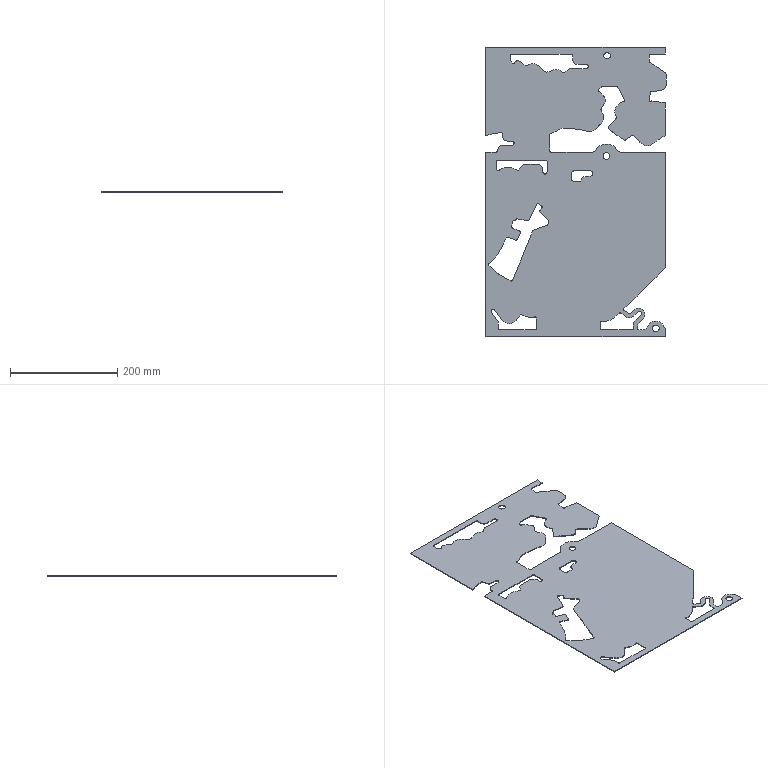Part | STEP file | gslz 2016.10.28-13_id190_x_t | 1 solid | 267 faces | box 337.305 x 540 x 1.25 mm | volume 189525 mm3 | cylinder 134 | plane 133 | commonest cylinder face diameters 4 x51 6 x13 20 x10 10 x9 30 x8 8 x7